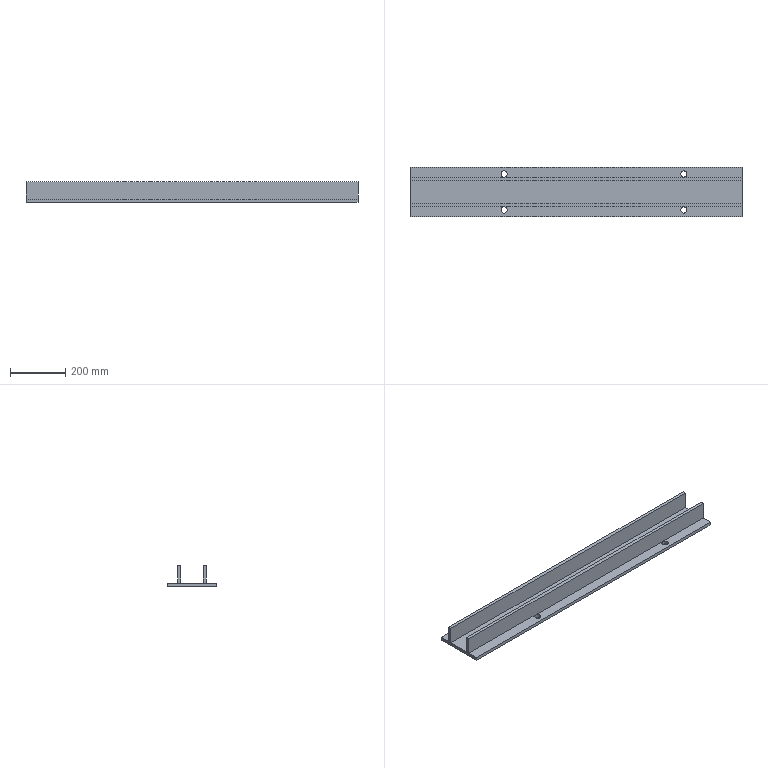Part | SolidWorks | features ICE 2, Extrusion 1, MirrorSolid 1, MoveFace 1 | 3 solids | 26 faces | box 1200 x 180 x 75.738 mm | volume 4409395 mm3 | plane 18 | cylinder 8 | commonest cylinder face diameters 22 x8
STEP:
#1=CARTESIAN_POINT('',(314.,65.,12.));
#2=VERTEX_POINT('',#1);
#3=CARTESIAN_POINT('',(336.,65.,12.));
#4=VERTEX_POINT('',#3);
#5=CARTESIAN_POINT('',(325.,65.,12.));
#6=DIRECTION('',(0.,0.,1.));
#7=DIRECTION('',(1.,0.,0.));
#8=AXIS2_PLACEMENT_3D('',#5,#6,#7);
#9=CIRCLE('',#8,11.);
#10=EDGE_CURVE('',#2,#4,#9,.T.);
#11=ORIENTED_EDGE('',*,*,#10,.T.);
#12=CARTESIAN_POINT('',(336.,65.,0.));
#13=VERTEX_POINT('',#12);
#14=CARTESIAN_POINT('',(336.,65.,12.));
#15=DIRECTION('',(0.,0.,-1.));
#16=VECTOR('',#15,1000.);
#17=LINE('',#14,#16);
#18=EDGE_CURVE('',#4,#13,#17,.T.);
#19=ORIENTED_EDGE('',*,*,#18,.T.);
#20=CARTESIAN_POINT('',(314.,65.,0.));
#21=VERTEX_POINT('',#20);
#22=CARTESIAN_POINT('',(325.,65.,0.));
#23=DIRECTION('',(0.,0.,1.));
#24=DIRECTION('',(1.,0.,0.));
#25=AXIS2_PLACEMENT_3D('',#22,#23,#24);
#26=CIRCLE('',#25,11.);
#27=EDGE_CURVE('',#21,#13,#26,.T.);
#28=ORIENTED_EDGE('',*,*,#27,.F.);
#29=CARTESIAN_POINT('',(314.,65.,12.));
#30=DIRECTION('',(0.,0.,-1.));
#31=VECTOR('',#30,1000.);
#32=LINE('',#29,#31);
#33=EDGE_CURVE('',#2,#21,#32,.T.);
#34=ORIENTED_EDGE('',*,*,#33,.F.);
#35=EDGE_LOOP('',(#11,#19,#28,#34));
#36=FACE_OUTER_BOUND('',#35,.T.);
#37=CARTESIAN_POINT('',(325.,65.,12.));
#38=DIRECTION('',(0.,0.,-1.));
#39=DIRECTION('',(-1.,0.,0.));
#40=AXIS2_PLACEMENT_3D('',#37,#38,#39);
#41=CYLINDRICAL_SURFACE('',#40,11.);
#42=ADVANCED_FACE('',(#36),#41,.F.);
#43=CARTESIAN_POINT('',(314.,-65.,12.));
#44=VERTEX_POINT('',#43);
#45=CARTESIAN_POINT('',(336.,-65.,12.));
#46=VERTEX_POINT('',#45);
#47=CARTESIAN_POINT('',(325.,-65.,12.));
#48=DIRECTION('',(0.,0.,1.));
#49=DIRECTION('',(1.,0.,0.));
#50=AXIS2_PLACEMENT_3D('',#47,#48,#49);
#51=CIRCLE('',#50,11.);
#52=EDGE_CURVE('',#44,#46,#51,.T.);
#53=ORIENTED_EDGE('',*,*,#52,.T.);
#54=CARTESIAN_POINT('',(336.,-65.,0.));
#55=VERTEX_POINT('',#54);
#56=CARTESIAN_POINT('',(336.,-65.,12.));
#57=DIRECTION('',(0.,0.,-1.));
#58=VECTOR('',#57,1000.);
#59=LINE('',#56,#58);
#60=EDGE_CURVE('',#46,#55,#59,.T.);
#61=ORIENTED_EDGE('',*,*,#60,.T.);
#62=CARTESIAN_POINT('',(314.,-65.,0.));
#63=VERTEX_POINT('',#62);
#64=CARTESIAN_POINT('',(325.,-65.,0.));
#65=DIRECTION('',(0.,0.,1.));
#66=DIRECTION('',(1.,0.,0.));
#67=AXIS2_PLACEMENT_3D('',#64,#65,#66);
#68=CIRCLE('',#67,11.);
#69=EDGE_CURVE('',#63,#55,#68,.T.);
#70=ORIENTED_EDGE('',*,*,#69,.F.);
#71=CARTESIAN_POINT('',(314.,-65.,12.));
#72=DIRECTION('',(0.,0.,-1.));
#73=VECTOR('',#72,1000.);
#74=LINE('',#71,#73);
#75=EDGE_CURVE('',#44,#63,#74,.T.);
#76=ORIENTED_EDGE('',*,*,#75,.F.);
#77=EDGE_LOOP('',(#53,#61,#70,#76));
#78=FACE_OUTER_BOUND('',#77,.T.);
#79=CARTESIAN_POINT('',(325.,-65.,12.));
#80=DIRECTION('',(0.,0.,-1.));
#81=DIRECTION('',(-1.,0.,0.));
#82=AXIS2_PLACEMENT_3D('',#79,#80,#81);
#83=CYLINDRICAL_SURFACE('',#82,11.);
#84=ADVANCED_FACE('',(#78),#83,.F.);
#85=CARTESIAN_POINT('',(-336.,65.,12.));
#86=VERTEX_POINT('',#85);
#87=CARTESIAN_POINT('',(-314.,65.,12.));
#88=VERTEX_POINT('',#87);
#89=CARTESIAN_POINT('',(-325.,65.,12.));
#90=DIRECTION('',(0.,0.,1.));
#91=DIRECTION('',(1.,0.,0.));
#92=AXIS2_PLACEMENT_3D('',#89,#90,#91);
#93=CIRCLE('',#92,11.);
#94=EDGE_CURVE('',#86,#88,#93,.T.);
#95=ORIENTED_EDGE('',*,*,#94,.T.);
#96=CARTESIAN_POINT('',(-314.,65.,0.));
#97=VERTEX_POINT('',#96);
#98=CARTESIAN_POINT('',(-314.,65.,12.));
#99=DIRECTION('',(0.,0.,-1.));
#100=VECTOR('',#99,1000.);
#101=LINE('',#98,#100);
#102=EDGE_CURVE('',#88,#97,#101,.T.);
#103=ORIENTED_EDGE('',*,*,#102,.T.);
#104=CARTESIAN_POINT('',(-336.,65.,0.));
#105=VERTEX_POINT('',#104);
#106=CARTESIAN_POINT('',(-325.,65.,0.));
#107=DIRECTION('',(0.,0.,1.));
#108=DIRECTION('',(1.,0.,0.));
#109=AXIS2_PLACEMENT_3D('',#106,#107,#108);
#110=CIRCLE('',#109,11.);
#111=EDGE_CURVE('',#105,#97,#110,.T.);
#112=ORIENTED_EDGE('',*,*,#111,.F.);
#113=CARTESIAN_POINT('',(-336.,65.,12.));
#114=DIRECTION('',(0.,0.,-1.));
#115=VECTOR('',#114,1000.);
#116=LINE('',#113,#115);
#117=EDGE_CURVE('',#86,#105,#116,.T.);
#118=ORIENTED_EDGE('',*,*,#117,.F.);
#119=EDGE_LOOP('',(#95,#103,#112,#118));
#120=FACE_OUTER_BOUND('',#119,.T.);
#121=CARTESIAN_POINT('',(-325.,65.,12.));
#122=DIRECTION('',(0.,0.,-1.));
#123=DIRECTION('',(-1.,0.,0.));
#124=AXIS2_PLACEMENT_3D('',#121,#122,#123);
#125=CYLINDRICAL_SURFACE('',#124,11.);
#126=ADVANCED_FACE('',(#120),#125,.F.);
#127=CARTESIAN_POINT('',(-336.,-65.,12.));
#128=VERTEX_POINT('',#127);
#129=CARTESIAN_POINT('',(-314.,-65.,12.));
#130=VERTEX_POINT('',#129);
#131=CARTESIAN_POINT('',(-325.,-65.,12.));
#132=DIRECTION('',(0.,0.,1.));
#133=DIRECTION('',(1.,0.,0.));
#134=AXIS2_PLACEMENT_3D('',#131,#132,#133);
#135=CIRCLE('',#134,11.);
#136=EDGE_CURVE('',#128,#130,#135,.T.);
#137=ORIENTED_EDGE('',*,*,#136,.T.);
#138=CARTESIAN_POINT('',(-314.,-65.,0.));
#139=VERTEX_POINT('',#138);
#140=CARTESIAN_POINT('',(-314.,-65.,12.));
#141=DIRECTION('',(0.,0.,-1.));
#142=VECTOR('',#141,1000.);
#143=LINE('',#140,#142);
#144=EDGE_CURVE('',#130,#139,#143,.T.);
#145=ORIENTED_EDGE('',*,*,#144,.T.);
#146=CARTESIAN_POINT('',(-336.,-65.,0.));
#147=VERTEX_POINT('',#146);
#148=CARTESIAN_POINT('',(-325.,-65.,0.));
#149=DIRECTION('',(0.,0.,1.));
#150=DIRECTION('',(1.,0.,0.));
#151=AXIS2_PLACEMENT_3D('',#148,#149,#150);
#152=CIRCLE('',#151,11.);
#153=EDGE_CURVE('',#147,#139,#152,.T.);
#154=ORIENTED_EDGE('',*,*,#153,.F.);
#155=CARTESIAN_POINT('',(-336.,-65.,12.));
#156=DIRECTION('',(0.,0.,-1.));
#157=VECTOR('',#156,1000.);
#158=LINE('',#155,#157);
#159=EDGE_CURVE('',#128,#147,#158,.T.);
#160=ORIENTED_EDGE('',*,*,#159,.F.);
#161=EDGE_LOOP('',(#137,#145,#154,#160));
#162=FACE_OUTER_BOUND('',#161,.T.);
#163=CARTESIAN_POINT('',(-325.,-65.,12.));
#164=DIRECTION('',(0.,0.,-1.));
#165=DIRECTION('',(-1.,0.,0.));
#166=AXIS2_PLACEMENT_3D('',#163,#164,#165);
#167=CYLINDRICAL_SURFACE('',#166,11.);
#168=ADVANCED_FACE('',(#162),#167,.F.);
#169=CARTESIAN_POINT('',(535.,-90.,12.));
#170=VERTEX_POINT('',#169);
#171=CARTESIAN_POINT('',(535.,90.,12.));
#172=VERTEX_POINT('',#171);
#173=CARTESIAN_POINT('',(535.,-90.,12.));
#174=DIRECTION('',(0.,1.,0.));
#175=VECTOR('',#174,1000.);
#176=LINE('',#173,#175);
#177=EDGE_CURVE('',#170,#172,#176,.T.);
#178=ORIENTED_EDGE('',*,*,#177,.T.);
#179=CARTESIAN_POINT('',(-665.,90.,12.));
#180=VERTEX_POINT('',#179);
#181=CARTESIAN_POINT('',(-365.,90.,12.));
#182=DIRECTION('',(-1.,0.,0.));
#183=VECTOR('',#182,1000.);
#184=LINE('',#181,#183);
#185=EDGE_CURVE('',#172,#180,#184,.T.);
#186=ORIENTED_EDGE('',*,*,#185,.T.);
#187=CARTESIAN_POINT('',(-665.,-90.,12.));
#188=VERTEX_POINT('',#187);
#189=CARTESIAN_POINT('',(-665.,90.,12.));
#190=DIRECTION('',(0.,-1.,0.));
#191=VECTOR('',#190,1000.);
#192=LINE('',#189,#191);
#193=EDGE_CURVE('',#180,#188,#192,.T.);
#194=ORIENTED_EDGE('',*,*,#193,.T.);
#195=CARTESIAN_POINT('',(-365.,-90.,12.));
#196=DIRECTION('',(1.,0.,0.));
#197=VECTOR('',#196,1000.);
#198=LINE('',#195,#197);
#199=EDGE_CURVE('',#188,#170,#198,.T.);
#200=ORIENTED_EDGE('',*,*,#199,.T.);
#201=EDGE_LOOP('',(#178,#186,#194,#200));
#202=FACE_OUTER_BOUND('',#201,.T.);
#203=ORIENTED_EDGE('',*,*,#136,.F.);
#204=CARTESIAN_POINT('',(-325.,-65.,12.));
#205=DIRECTION('',(0.,0.,1.));
#206=DIRECTION('',(1.,0.,0.));
#207=AXIS2_PLACEMENT_3D('',#204,#205,#206);
#208=CIRCLE('',#207,11.);
#209=EDGE_CURVE('',#130,#128,#208,.T.);
#210=ORIENTED_EDGE('',*,*,#209,.F.);
#211=EDGE_LOOP('',(#203,#210));
#212=FACE_BOUND('',#211,.T.);
#213=ORIENTED_EDGE('',*,*,#94,.F.);
#214=CARTESIAN_POINT('',(-325.,65.,12.));
#215=DIRECTION('',(0.,0.,1.));
#216=DIRECTION('',(1.,0.,0.));
#217=AXIS2_PLACEMENT_3D('',#214,#215,#216);
#218=CIRCLE('',#217,11.);
#219=EDGE_CURVE('',#88,#86,#218,.T.);
#220=ORIENTED_EDGE('',*,*,#219,.F.);
#221=EDGE_LOOP('',(#213,#220));
#222=FACE_BOUND('',#221,.T.);
#223=ORIENTED_EDGE('',*,*,#52,.F.);
#224=CARTESIAN_POINT('',(325.,-65.,12.));
#225=DIRECTION('',(0.,0.,1.));
#226=DIRECTION('',(1.,0.,0.));
#227=AXIS2_PLACEMENT_3D('',#224,#225,#226);
#228=CIRCLE('',#227,11.);
#229=EDGE_CURVE('',#46,#44,#228,.T.);
#230=ORIENTED_EDGE('',*,*,#229,.F.);
#231=EDGE_LOOP('',(#223,#230));
#232=FACE_BOUND('',#231,.T.);
#233=ORIENTED_EDGE('',*,*,#10,.F.);
#234=CARTESIAN_POINT('',(325.,65.,12.));
#235=DIRECTION('',(0.,0.,1.));
#236=DIRECTION('',(1.,0.,0.));
#237=AXIS2_PLACEMENT_3D('',#234,#235,#236);
#238=CIRCLE('',#237,11.);
#239=EDGE_CURVE('',#4,#2,#238,.T.);
#240=ORIENTED_EDGE('',*,*,#239,.F.);
#241=EDGE_LOOP('',(#233,#240));
#242=FACE_BOUND('',#241,.T.);
#243=CARTESIAN_POINT('',(535.,90.,12.));
#244=DIRECTION('',(0.,0.,-1.));
#245=DIRECTION('',(-1.,0.,0.));
#246=AXIS2_PLACEMENT_3D('',#243,#244,#245);
#247=PLANE('',#246);
#248=ADVANCED_FACE('',(#202,#212,#222,#232,#242),#247,.F.);
#249=ORIENTED_EDGE('',*,*,#69,.T.);
#250=CARTESIAN_POINT('',(325.,-65.,0.));
#251=DIRECTION('',(0.,0.,1.));
#252=DIRECTION('',(1.,0.,0.));
#253=AXIS2_PLACEMENT_3D('',#250,#251,#252);
#254=CIRCLE('',#253,11.);
#255=EDGE_CURVE('',#55,#63,#254,.T.);
#256=ORIENTED_EDGE('',*,*,#255,.T.);
#257=EDGE_LOOP('',(#249,#256));
#258=FACE_BOUND('',#257,.T.);
#259=ORIENTED_EDGE('',*,*,#153,.T.);
#260=CARTESIAN_POINT('',(-325.,-65.,0.));
#261=DIRECTION('',(0.,0.,1.));
#262=DIRECTION('',(1.,0.,0.));
#263=AXIS2_PLACEMENT_3D('',#260,#261,#262);
#264=CIRCLE('',#263,11.);
#265=EDGE_CURVE('',#139,#147,#264,.T.);
#266=ORIENTED_EDGE('',*,*,#265,.T.);
#267=EDGE_LOOP('',(#259,#266));
#268=FACE_BOUND('',#267,.T.);
#269=CARTESIAN_POINT('',(535.,-90.,0.));
#270=VERTEX_POINT('',#269);
#271=CARTESIAN_POINT('',(535.,90.,0.));
#272=VERTEX_POINT('',#271);
#273=CARTESIAN_POINT('',(535.,-90.,0.));
#274=DIRECTION('',(0.,1.,0.));
#275=VECTOR('',#274,1000.);
#276=LINE('',#273,#275);
#277=EDGE_CURVE('',#270,#272,#276,.T.);
#278=ORIENTED_EDGE('',*,*,#277,.F.);
#279=CARTESIAN_POINT('',(-665.,-90.,0.));
#280=VERTEX_POINT('',#279);
#281=CARTESIAN_POINT('',(-365.,-90.,0.));
#282=DIRECTION('',(1.,0.,0.));
#283=VECTOR('',#282,1000.);
#284=LINE('',#281,#283);
#285=EDGE_CURVE('',#280,#270,#284,.T.);
#286=ORIENTED_EDGE('',*,*,#285,.F.);
#287=CARTESIAN_POINT('',(-665.,90.,0.));
#288=VERTEX_POINT('',#287);
#289=CARTESIAN_POINT('',(-665.,90.,0.));
#290=DIRECTION('',(0.,-1.,0.));
#291=VECTOR('',#290,1000.);
#292=LINE('',#289,#291);
#293=EDGE_CURVE('',#288,#280,#292,.T.);
#294=ORIENTED_EDGE('',*,*,#293,.F.);
#295=CARTESIAN_POINT('',(-365.,90.,0.));
#296=DIRECTION('',(-1.,0.,0.));
#297=VECTOR('',#296,1000.);
#298=LINE('',#295,#297);
#299=EDGE_CURVE('',#272,#288,#298,.T.);
#300=ORIENTED_EDGE('',*,*,#299,.F.);
#301=EDGE_LOOP('',(#278,#286,#294,#300));
#302=FACE_OUTER_BOUND('',#301,.T.);
#303=ORIENTED_EDGE('',*,*,#111,.T.);
#304=CARTESIAN_POINT('',(-325.,65.,0.));
#305=DIRECTION('',(0.,0.,1.));
#306=DIRECTION('',(1.,0.,0.));
#307=AXIS2_PLACEMENT_3D('',#304,#305,#306);
#308=CIRCLE('',#307,11.);
#309=EDGE_CURVE('',#97,#105,#308,.T.);
#310=ORIENTED_EDGE('',*,*,#309,.T.);
#311=EDGE_LOOP('',(#303,#310));
#312=FACE_BOUND('',#311,.T.);
#313=ORIENTED_EDGE('',*,*,#27,.T.);
#314=CARTESIAN_POINT('',(325.,65.,0.));
#315=DIRECTION('',(0.,0.,1.));
#316=DIRECTION('',(1.,0.,0.));
#317=AXIS2_PLACEMENT_3D('',#314,#315,#316);
#318=CIRCLE('',#317,11.);
#319=EDGE_CURVE('',#13,#21,#318,.T.);
#320=ORIENTED_EDGE('',*,*,#319,.T.);
#321=EDGE_LOOP('',(#313,#320));
#322=FACE_BOUND('',#321,.T.);
#323=CARTESIAN_POINT('',(535.,90.,0.));
#324=DIRECTION('',(0.,0.,-1.));
#325=DIRECTION('',(-1.,0.,0.));
#326=AXIS2_PLACEMENT_3D('',#323,#324,#325);
#327=PLANE('',#326);
#328=ADVANCED_FACE('',(#258,#268,#302,#312,#322),#327,.T.);
#329=ORIENTED_EDGE('',*,*,#277,.T.);
#330=CARTESIAN_POINT('',(535.,90.,12.));
#331=DIRECTION('',(0.,0.,-1.));
#332=VECTOR('',#331,1000.);
#333=LINE('',#330,#332);
#334=EDGE_CURVE('',#172,#272,#333,.T.);
#335=ORIENTED_EDGE('',*,*,#334,.F.);
#336=ORIENTED_EDGE('',*,*,#177,.F.);
#337=CARTESIAN_POINT('',(535.,-90.,12.));
#338=DIRECTION('',(0.,0.,-1.));
#339=VECTOR('',#338,1000.);
#340=LINE('',#337,#339);
#341=EDGE_CURVE('',#170,#270,#340,.T.);
#342=ORIENTED_EDGE('',*,*,#341,.T.);
#343=EDGE_LOOP('',(#329,#335,#336,#342));
#344=FACE_OUTER_BOUND('',#343,.T.);
#345=CARTESIAN_POINT('',(535.,-90.,12.));
#346=DIRECTION('',(-1.,0.,0.));
#347=DIRECTION('',(0.,0.,1.));
#348=AXIS2_PLACEMENT_3D('',#345,#346,#347);
#349=PLANE('',#348);
#350=ADVANCED_FACE('',(#344),#349,.F.);
#351=ORIENTED_EDGE('',*,*,#299,.T.);
#352=CARTESIAN_POINT('',(-665.,90.,12.));
#353=DIRECTION('',(0.,0.,-1.));
#354=VECTOR('',#353,1000.);
#355=LINE('',#352,#354);
#356=EDGE_CURVE('',#180,#288,#355,.T.);
#357=ORIENTED_EDGE('',*,*,#356,.F.);
#358=ORIENTED_EDGE('',*,*,#185,.F.);
#359=ORIENTED_EDGE('',*,*,#334,.T.);
#360=EDGE_LOOP('',(#351,#357,#358,#359));
#361=FACE_OUTER_BOUND('',#360,.T.);
#362=CARTESIAN_POINT('',(-365.,90.,12.));
#363=DIRECTION('',(0.,-1.,0.));
#364=DIRECTION('',(0.,0.,-1.));
#365=AXIS2_PLACEMENT_3D('',#362,#363,#364);
#366=PLANE('',#365);
#367=ADVANCED_FACE('',(#361),#366,.F.);
#368=ORIENTED_EDGE('',*,*,#293,.T.);
#369=CARTESIAN_POINT('',(-665.,-90.,12.));
#370=DIRECTION('',(0.,0.,-1.));
#371=VECTOR('',#370,1000.);
#372=LINE('',#369,#371);
#373=EDGE_CURVE('',#188,#280,#372,.T.);
#374=ORIENTED_EDGE('',*,*,#373,.F.);
#375=ORIENTED_EDGE('',*,*,#193,.F.);
#376=ORIENTED_EDGE('',*,*,#356,.T.);
#377=EDGE_LOOP('',(#368,#374,#375,#376));
#378=FACE_OUTER_BOUND('',#377,.T.);
#379=CARTESIAN_POINT('',(-665.,-90.,12.));
#380=DIRECTION('',(1.,0.,0.));
#381=DIRECTION('',(0.,0.,-1.));
#382=AXIS2_PLACEMENT_3D('',#379,#380,#381);
#383=PLANE('',#382);
#384=ADVANCED_FACE('',(#378),#383,.F.);
#385=ORIENTED_EDGE('',*,*,#285,.T.);
#386=ORIENTED_EDGE('',*,*,#341,.F.);
#387=ORIENTED_EDGE('',*,*,#199,.F.);
#388=ORIENTED_EDGE('',*,*,#373,.T.);
#389=EDGE_LOOP('',(#385,#386,#387,#388));
#390=FACE_OUTER_BOUND('',#389,.T.);
#391=CARTESIAN_POINT('',(-365.,-90.,12.));
#392=DIRECTION('',(0.,1.,0.));
#393=DIRECTION('',(0.,0.,1.));
#394=AXIS2_PLACEMENT_3D('',#391,#392,#393);
#395=PLANE('',#394);
#396=ADVANCED_FACE('',(#390),#395,.F.);
#397=ORIENTED_EDGE('',*,*,#144,.F.);
#398=ORIENTED_EDGE('',*,*,#209,.T.);
#399=ORIENTED_EDGE('',*,*,#159,.T.);
#400=ORIENTED_EDGE('',*,*,#265,.F.);
#401=EDGE_LOOP('',(#397,#398,#399,#400));
#402=FACE_OUTER_BOUND('',#401,.T.);
#403=CARTESIAN_POINT('',(-325.,-65.,12.));
#404=DIRECTION('',(0.,0.,-1.));
#405=DIRECTION('',(-1.,0.,0.));
#406=AXIS2_PLACEMENT_3D('',#403,#404,#405);
#407=CYLINDRICAL_SURFACE('',#406,11.);
#408=ADVANCED_FACE('',(#402),#407,.F.);
#409=ORIENTED_EDGE('',*,*,#102,.F.);
#410=ORIENTED_EDGE('',*,*,#219,.T.);
#411=ORIENTED_EDGE('',*,*,#117,.T.);
#412=ORIENTED_EDGE('',*,*,#309,.F.);
#413=EDGE_LOOP('',(#409,#410,#411,#412));
#414=FACE_OUTER_BOUND('',#413,.T.);
#415=CARTESIAN_POINT('',(-325.,65.,12.));
#416=DIRECTION('',(0.,0.,-1.));
#417=DIRECTION('',(-1.,0.,0.));
#418=AXIS2_PLACEMENT_3D('',#415,#416,#417);
#419=CYLINDRICAL_SURFACE('',#418,11.);
#420=ADVANCED_FACE('',(#414),#419,.F.);
#421=ORIENTED_EDGE('',*,*,#60,.F.);
#422=ORIENTED_EDGE('',*,*,#229,.T.);
#423=ORIENTED_EDGE('',*,*,#75,.T.);
#424=ORIENTED_EDGE('',*,*,#255,.F.);
#425=EDGE_LOOP('',(#421,#422,#423,#424));
#426=FACE_OUTER_BOUND('',#425,.T.);
#427=CARTESIAN_POINT('',(325.,-65.,12.));
#428=DIRECTION('',(0.,0.,-1.));
#429=DIRECTION('',(-1.,0.,0.));
#430=AXIS2_PLACEMENT_3D('',#427,#428,#429);
#431=CYLINDRICAL_SURFACE('',#430,11.);
#432=ADVANCED_FACE('',(#426),#431,.F.);
#433=ORIENTED_EDGE('',*,*,#18,.F.);
#434=ORIENTED_EDGE('',*,*,#239,.T.);
#435=ORIENTED_EDGE('',*,*,#33,.T.);
#436=ORIENTED_EDGE('',*,*,#319,.F.);
#437=EDGE_LOOP('',(#433,#434,#435,#436));
#438=FACE_OUTER_BOUND('',#437,.T.);
#439=CARTESIAN_POINT('',(325.,65.,12.));
#440=DIRECTION('',(0.,0.,-1.));
#441=DIRECTION('',(-1.,0.,0.));
#442=AXIS2_PLACEMENT_3D('',#439,#440,#441);
#443=CYLINDRICAL_SURFACE('',#442,11.);
#444=ADVANCED_FACE('',(#438),#443,.F.);
#445=CLOSED_SHELL('',(#42,#84,#126,#168,#248,#328,#350,#367,#384,#396,#408,#420,#432,#444));
#446=MANIFOLD_SOLID_BREP('',#445);
#447=CARTESIAN_POINT('',(535.,-40.,12.));
#448=VERTEX_POINT('',#447);
#449=CARTESIAN_POINT('',(-665.,-40.,12.));
#450=VERTEX_POINT('',#449);
#451=CARTESIAN_POINT('',(-365.,-40.,12.));
#452=DIRECTION('',(-1.,0.,0.));
#453=VECTOR('',#452,1000.);
#454=LINE('',#451,#453);
#455=EDGE_CURVE('',#448,#450,#454,.T.);
#456=ORIENTED_EDGE('',*,*,#455,.F.);
#457=CARTESIAN_POINT('',(535.,-52.,12.));
#458=VERTEX_POINT('',#457);
#459=CARTESIAN_POINT('',(535.,-52.,12.));
#460=DIRECTION('',(0.,1.,0.));
#461=VECTOR('',#460,1000.);
#462=LINE('',#459,#461);
#463=EDGE_CURVE('',#458,#448,#462,.T.);
#464=ORIENTED_EDGE('',*,*,#463,.F.);
#465=CARTESIAN_POINT('',(-665.,-52.,12.));
#466=VERTEX_POINT('',#465);
#467=CARTESIAN_POINT('',(-365.,-52.,12.));
#468=DIRECTION('',(-1.,0.,0.));
#469=VECTOR('',#468,1000.);
#470=LINE('',#467,#469);
#471=EDGE_CURVE('',#458,#466,#470,.T.);
#472=ORIENTED_EDGE('',*,*,#471,.T.);
#473=CARTESIAN_POINT('',(-665.,-52.,12.));
#474=DIRECTION('',(0.,1.,0.));
#475=VECTOR('',#474,1000.);
#476=LINE('',#473,#475);
#477=EDGE_CURVE('',#466,#450,#476,.T.);
#478=ORIENTED_EDGE('',*,*,#477,.T.);
#479=EDGE_LOOP('',(#456,#464,#472,#478));
#480=FACE_OUTER_BOUND('',#479,.T.);
#481=CARTESIAN_POINT('',(-365.,-52.,12.));
#482=DIRECTION('',(0.,0.,1.));
#483=DIRECTION('',(1.,0.,0.));
#484=AXIS2_PLACEMENT_3D('',#481,#482,#483);
#485=PLANE('',#484);
#486=ADVANCED_FACE('',(#480),#485,.F.);
#487=CARTESIAN_POINT('',(-665.,-40.,75.738));
#488=VERTEX_POINT('',#487);
#489=CARTESIAN_POINT('',(-665.,-40.,75.738));
#490=DIRECTION('',(0.,0.,1.));
#491=VECTOR('',#490,1000.);
#492=LINE('',#489,#491);
#493=EDGE_CURVE('',#450,#488,#492,.T.);
#494=ORIENTED_EDGE('',*,*,#493,.F.);
#495=ORIENTED_EDGE('',*,*,#477,.F.);
#496=CARTESIAN_POINT('',(-665.,-52.,75.738));
#497=VERTEX_POINT('',#496);
#498=CARTESIAN_POINT('',(-665.,-52.,75.738));
#499=DIRECTION('',(0.,0.,1.));
#500=VECTOR('',#499,1000.);
#501=LINE('',#498,#500);
#502=EDGE_CURVE('',#466,#497,#501,.T.);
#503=ORIENTED_EDGE('',*,*,#502,.T.);
#504=CARTESIAN_POINT('',(-665.,-52.,75.738));
#505=DIRECTION('',(0.,1.,0.));
#506=VECTOR('',#505,1000.);
#507=LINE('',#504,#506);
#508=EDGE_CURVE('',#497,#488,#507,.T.);
#509=ORIENTED_EDGE('',*,*,#508,.T.);
#510=EDGE_LOOP('',(#494,#495,#503,#509));
#511=FACE_OUTER_BOUND('',#510,.T.);
#512=CARTESIAN_POINT('',(-665.,-52.,75.738));
#513=DIRECTION('',(1.,0.,0.));
#514=DIRECTION('',(0.,0.,-1.));
#515=AXIS2_PLACEMENT_3D('',#512,#513,#514);
#516=PLANE('',#515);
#517=ADVANCED_FACE('',(#511),#516,.F.);
#518=CARTESIAN_POINT('',(535.,-52.,75.738));
#519=VERTEX_POINT('',#518);
#520=CARTESIAN_POINT('',(1337.,-52.,75.738));
#521=DIRECTION('',(1.,0.,0.));
#522=VECTOR('',#521,1000.);
#523=LINE('',#520,#522);
#524=EDGE_CURVE('',#497,#519,#523,.T.);
#525=ORIENTED_EDGE('',*,*,#524,.T.);
#526=CARTESIAN_POINT('',(535.,-40.,75.738));
#527=VERTEX_POINT('',#526);
#528=CARTESIAN_POINT('',(535.,-52.,75.738));
#529=DIRECTION('',(0.,1.,0.));
#530=VECTOR('',#529,1000.);
#531=LINE('',#528,#530);
#532=EDGE_CURVE('',#519,#527,#531,.T.);
#533=ORIENTED_EDGE('',*,*,#532,.T.);
#534=CARTESIAN_POINT('',(1337.,-40.,75.738));
#535=DIRECTION('',(1.,0.,0.));
#536=VECTOR('',#535,1000.);
#537=LINE('',#534,#536);
#538=EDGE_CURVE('',#488,#527,#537,.T.);
#539=ORIENTED_EDGE('',*,*,#538,.F.);
#540=ORIENTED_EDGE('',*,*,#508,.F.);
#541=EDGE_LOOP('',(#525,#533,#539,#540));
#542=FACE_OUTER_BOUND('',#541,.T.);
#543=CARTESIAN_POINT('',(1337.,-52.,75.738));
#544=DIRECTION('',(0.,0.,-1.));
#545=DIRECTION('',(-1.,0.,0.));
#546=AXIS2_PLACEMENT_3D('',#543,#544,#545);
#547=PLANE('',#546);
#548=ADVANCED_FACE('',(#542),#547,.F.);
#549=CARTESIAN_POINT('',(535.,-40.,12.));
#550=DIRECTION('',(0.,0.,-1.));
#551=VECTOR('',#550,1000.);
#552=LINE('',#549,#551);
#553=EDGE_CURVE('',#527,#448,#552,.T.);
#554=ORIENTED_EDGE('',*,*,#553,.F.);
#555=ORIENTED_EDGE('',*,*,#532,.F.);
#556=CARTESIAN_POINT('',(535.,-52.,12.));
#557=DIRECTION('',(0.,0.,-1.));
#558=VECTOR('',#557,1000.);
#559=LINE('',#556,#558);
#560=EDGE_CURVE('',#519,#458,#559,.T.);
#561=ORIENTED_EDGE('',*,*,#560,.T.);
#562=ORIENTED_EDGE('',*,*,#463,.T.);
#563=EDGE_LOOP('',(#554,#555,#561,#562));
#564=FACE_OUTER_BOUND('',#563,.T.);
#565=CARTESIAN_POINT('',(535.,-52.,12.));
#566=DIRECTION('',(-1.,0.,0.));
#567=DIRECTION('',(0.,0.,1.));
#568=AXIS2_PLACEMENT_3D('',#565,#566,#567);
#569=PLANE('',#568);
#570=ADVANCED_FACE('',(#564),#569,.F.);
#571=ORIENTED_EDGE('',*,*,#560,.F.);
#572=ORIENTED_EDGE('',*,*,#524,.F.);
#573=ORIENTED_EDGE('',*,*,#502,.F.);
#574=ORIENTED_EDGE('',*,*,#471,.F.);
#575=EDGE_LOOP('',(#571,#572,#573,#574));
#576=FACE_OUTER_BOUND('',#575,.T.);
#577=CARTESIAN_POINT('',(535.,-52.,12.));
#578=DIRECTION('',(0.,1.,0.));
#579=DIRECTION('',(0.,0.,-1.));
#580=AXIS2_PLACEMENT_3D('',#577,#578,#579);
#581=PLANE('',#580);
#582=ADVANCED_FACE('',(#576),#581,.F.);
#583=ORIENTED_EDGE('',*,*,#538,.T.);
#584=ORIENTED_EDGE('',*,*,#553,.T.);
#585=ORIENTED_EDGE('',*,*,#455,.T.);
#586=ORIENTED_EDGE('',*,*,#493,.T.);
#587=EDGE_LOOP('',(#583,#584,#585,#586));
#588=FACE_OUTER_BOUND('',#587,.T.);
#589=CARTESIAN_POINT('',(535.,-40.,12.));
#590=DIRECTION('',(0.,1.,0.));
#591=DIRECTION('',(0.,0.,-1.));
#592=AXIS2_PLACEMENT_3D('',#589,#590,#591);
#593=PLANE('',#592);
#594=ADVANCED_FACE('',(#588),#593,.T.);
#595=CLOSED_SHELL('',(#486,#517,#548,#570,#582,#594));
#596=MANIFOLD_SOLID_BREP('',#595);
#597=CARTESIAN_POINT('',(535.,40.,12.));
#598=VERTEX_POINT('',#597);
#599=CARTESIAN_POINT('',(-665.,40.,12.));
#600=VERTEX_POINT('',#599);
#601=CARTESIAN_POINT('',(-365.,40.,12.));
#602=DIRECTION('',(-1.,0.,0.));
#603=VECTOR('',#602,1000.);
#604=LINE('',#601,#603);
#605=EDGE_CURVE('',#598,#600,#604,.T.);
#606=ORIENTED_EDGE('',*,*,#605,.T.);
#607=CARTESIAN_POINT('',(-665.,52.,12.));
#608=VERTEX_POINT('',#607);
#609=CARTESIAN_POINT('',(-665.,52.,12.));
#610=DIRECTION('',(0.,-1.,0.));
#611=VECTOR('',#610,1000.);
#612=LINE('',#609,#611);
#613=EDGE_CURVE('',#608,#600,#612,.T.);
#614=ORIENTED_EDGE('',*,*,#613,.F.);
#615=CARTESIAN_POINT('',(535.,52.,12.));
#616=VERTEX_POINT('',#615);
#617=CARTESIAN_POINT('',(-365.,52.,12.));
#618=DIRECTION('',(-1.,0.,0.));
#619=VECTOR('',#618,1000.);
#620=LINE('',#617,#619);
#621=EDGE_CURVE('',#616,#608,#620,.T.);
#622=ORIENTED_EDGE('',*,*,#621,.F.);
#623=CARTESIAN_POINT('',(535.,52.,12.));
#624=DIRECTION('',(0.,-1.,0.));
#625=VECTOR('',#624,1000.);
#626=LINE('',#623,#625);
#627=EDGE_CURVE('',#616,#598,#626,.T.);
#628=ORIENTED_EDGE('',*,*,#627,.T.);
#629=EDGE_LOOP('',(#606,#614,#622,#628));
#630=FACE_OUTER_BOUND('',#629,.T.);
#631=CARTESIAN_POINT('',(-365.,52.,12.));
#632=DIRECTION('',(0.,0.,1.));
#633=DIRECTION('',(1.,0.,0.));
#634=AXIS2_PLACEMENT_3D('',#631,#632,#633);
#635=PLANE('',#634);
#636=ADVANCED_FACE('',(#630),#635,.F.);
#637=CARTESIAN_POINT('',(-665.,40.,75.738));
#638=VERTEX_POINT('',#637);
#639=CARTESIAN_POINT('',(-665.,40.,12.));
#640=DIRECTION('',(0.,0.,1.));
#641=VECTOR('',#640,1000.);
#642=LINE('',#639,#641);
#643=EDGE_CURVE('',#600,#638,#642,.T.);
#644=ORIENTED_EDGE('',*,*,#643,.T.);
#645=CARTESIAN_POINT('',(-665.,52.,75.738));
#646=VERTEX_POINT('',#645);
#647=CARTESIAN_POINT('',(-665.,52.,75.738));
#648=DIRECTION('',(0.,-1.,0.));
#649=VECTOR('',#648,1000.);
#650=LINE('',#647,#649);
#651=EDGE_CURVE('',#646,#638,#650,.T.);
#652=ORIENTED_EDGE('',*,*,#651,.F.);
#653=CARTESIAN_POINT('',(-665.,52.,12.));
#654=DIRECTION('',(0.,0.,1.));
#655=VECTOR('',#654,1000.);
#656=LINE('',#653,#655);
#657=EDGE_CURVE('',#608,#646,#656,.T.);
#658=ORIENTED_EDGE('',*,*,#657,.F.);
#659=ORIENTED_EDGE('',*,*,#613,.T.);
#660=EDGE_LOOP('',(#644,#652,#658,#659));
#661=FACE_OUTER_BOUND('',#660,.T.);
#662=CARTESIAN_POINT('',(-665.,52.,75.738));
#663=DIRECTION('',(1.,0.,0.));
#664=DIRECTION('',(0.,0.,-1.));
#665=AXIS2_PLACEMENT_3D('',#662,#663,#664);
#666=PLANE('',#665);
#667=ADVANCED_FACE('',(#661),#666,.F.);
#668=CARTESIAN_POINT('',(535.,40.,75.738));
#669=VERTEX_POINT('',#668);
#670=CARTESIAN_POINT('',(1337.,40.,75.738));
#671=DIRECTION('',(1.,0.,0.));
#672=VECTOR('',#671,1000.);
#673=LINE('',#670,#672);
#674=EDGE_CURVE('',#638,#669,#673,.T.);
#675=ORIENTED_EDGE('',*,*,#674,.T.);
#676=CARTESIAN_POINT('',(535.,52.,75.738));
#677=VERTEX_POINT('',#676);
#678=CARTESIAN_POINT('',(535.,52.,75.738));
#679=DIRECTION('',(0.,1.,0.));
#680=VECTOR('',#679,1000.);
#681=LINE('',#678,#680);
#682=EDGE_CURVE('',#669,#677,#681,.T.);
#683=ORIENTED_EDGE('',*,*,#682,.T.);
#684=CARTESIAN_POINT('',(1337.,52.,75.738));
#685=DIRECTION('',(1.,0.,0.));
#686=VECTOR('',#685,1000.);
#687=LINE('',#684,#686);
#688=EDGE_CURVE('',#646,#677,#687,.T.);
#689=ORIENTED_EDGE('',*,*,#688,.F.);
#690=ORIENTED_EDGE('',*,*,#651,.T.);
#691=EDGE_LOOP('',(#675,#683,#689,#690));
#692=FACE_OUTER_BOUND('',#691,.T.);
#693=CARTESIAN_POINT('',(1337.,52.,75.738));
#694=DIRECTION('',(0.,0.,-1.));
#695=DIRECTION('',(-1.,0.,0.));
#696=AXIS2_PLACEMENT_3D('',#693,#694,#695);
#697=PLANE('',#696);
#698=ADVANCED_FACE('',(#692),#697,.F.);
#699=CARTESIAN_POINT('',(535.,40.,12.));
#700=DIRECTION('',(0.,0.,-1.));
#701=VECTOR('',#700,1000.);
#702=LINE('',#699,#701);
#703=EDGE_CURVE('',#669,#598,#702,.T.);
#704=ORIENTED_EDGE('',*,*,#703,.T.);
#705=ORIENTED_EDGE('',*,*,#627,.F.);
#706=CARTESIAN_POINT('',(535.,52.,12.));
#707=DIRECTION('',(0.,0.,-1.));
#708=VECTOR('',#707,1000.);
#709=LINE('',#706,#708);
#710=EDGE_CURVE('',#677,#616,#709,.T.);
#711=ORIENTED_EDGE('',*,*,#710,.F.);
#712=ORIENTED_EDGE('',*,*,#682,.F.);
#713=EDGE_LOOP('',(#704,#705,#711,#712));
#714=FACE_OUTER_BOUND('',#713,.T.);
#715=CARTESIAN_POINT('',(535.,52.,12.));
#716=DIRECTION('',(-1.,0.,0.));
#717=DIRECTION('',(0.,0.,1.));
#718=AXIS2_PLACEMENT_3D('',#715,#716,#717);
#719=PLANE('',#718);
#720=ADVANCED_FACE('',(#714),#719,.F.);
#721=ORIENTED_EDGE('',*,*,#688,.T.);
#722=ORIENTED_EDGE('',*,*,#710,.T.);
#723=ORIENTED_EDGE('',*,*,#621,.T.);
#724=ORIENTED_EDGE('',*,*,#657,.T.);
#725=EDGE_LOOP('',(#721,#722,#723,#724));
#726=FACE_OUTER_BOUND('',#725,.T.);
#727=CARTESIAN_POINT('',(535.,52.,12.));
#728=DIRECTION('',(0.,-1.,0.));
#729=DIRECTION('',(0.,0.,-1.));
#730=AXIS2_PLACEMENT_3D('',#727,#728,#729);
#731=PLANE('',#730);
#732=ADVANCED_FACE('',(#726),#731,.F.);
#733=ORIENTED_EDGE('',*,*,#703,.F.);
#734=ORIENTED_EDGE('',*,*,#674,.F.);
#735=ORIENTED_EDGE('',*,*,#643,.F.);
#736=ORIENTED_EDGE('',*,*,#605,.F.);
#737=EDGE_LOOP('',(#733,#734,#735,#736));
#738=FACE_OUTER_BOUND('',#737,.T.);
#739=CARTESIAN_POINT('',(535.,40.,12.));
#740=DIRECTION('',(0.,-1.,0.));
#741=DIRECTION('',(0.,0.,-1.));
#742=AXIS2_PLACEMENT_3D('',#739,#740,#741);
#743=PLANE('',#742);
#744=ADVANCED_FACE('',(#738),#743,.T.);
#745=CLOSED_SHELL('',(#636,#667,#698,#720,#732,#744));
#746=MANIFOLD_SOLID_BREP('',#745);
#747=CARTESIAN_POINT('',(0.,0.,0.));
#748=DIRECTION('',(0.,0.,1.));
#749=DIRECTION('',(1.,0.,0.));
#750=AXIS2_PLACEMENT_3D('',#747,#748,#749);
#751=(LENGTH_UNIT()NAMED_UNIT(*)SI_UNIT(.MILLI.,.METRE.));
#752=UNCERTAINTY_MEASURE_WITH_UNIT(LENGTH_MEASURE(0.00001),#751,'','');
#753=(NAMED_UNIT(*)PLANE_ANGLE_UNIT()SI_UNIT($,.RADIAN.));
#754=(NAMED_UNIT(*)SI_UNIT($,.STERADIAN.)SOLID_ANGLE_UNIT());
#755=(GEOMETRIC_REPRESENTATION_CONTEXT(3)GLOBAL_UNCERTAINTY_ASSIGNED_CONTEXT((#752))GLOBAL_UNIT_ASSIGNED_CONTEXT((#751,#753,#754))REPRESENTATION_CONTEXT('',''));
#756=ADVANCED_BREP_SHAPE_REPRESENTATION('',(#446,#596,#746,#750),#755);